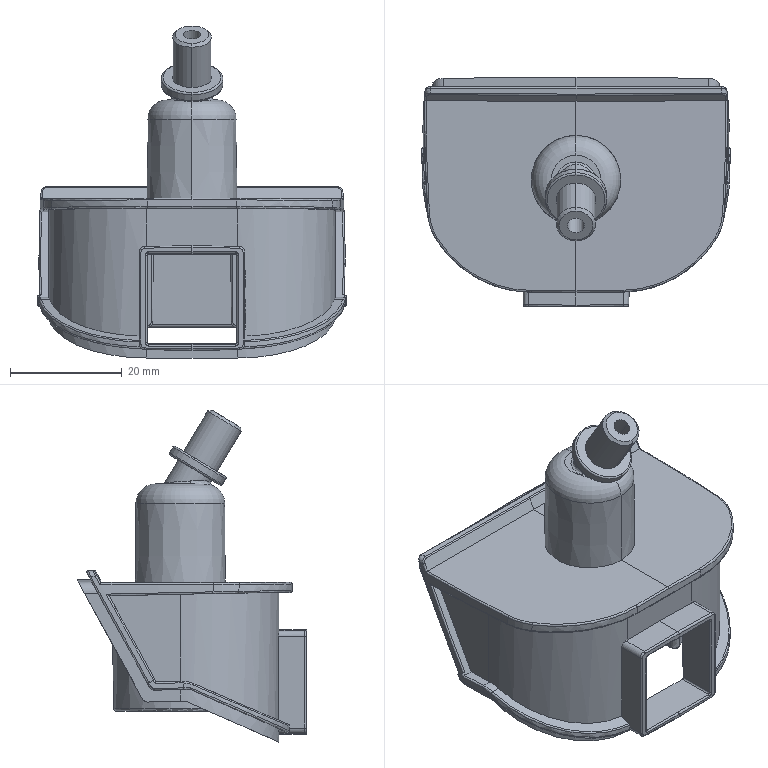Part | STEP file | lll_id46_x_t | 1 solid | 361 faces | box 55.309 x 41.141 x 59.468 mm | volume 14807 mm3 | plane 146 | spline 110 | cylinder 73 | torus 18 | cone 14 | commonest cylinder face diameters 0.602 x35 2.008 x12 1.004 x5 3.012 x4 7.028 x4 35.14 x4